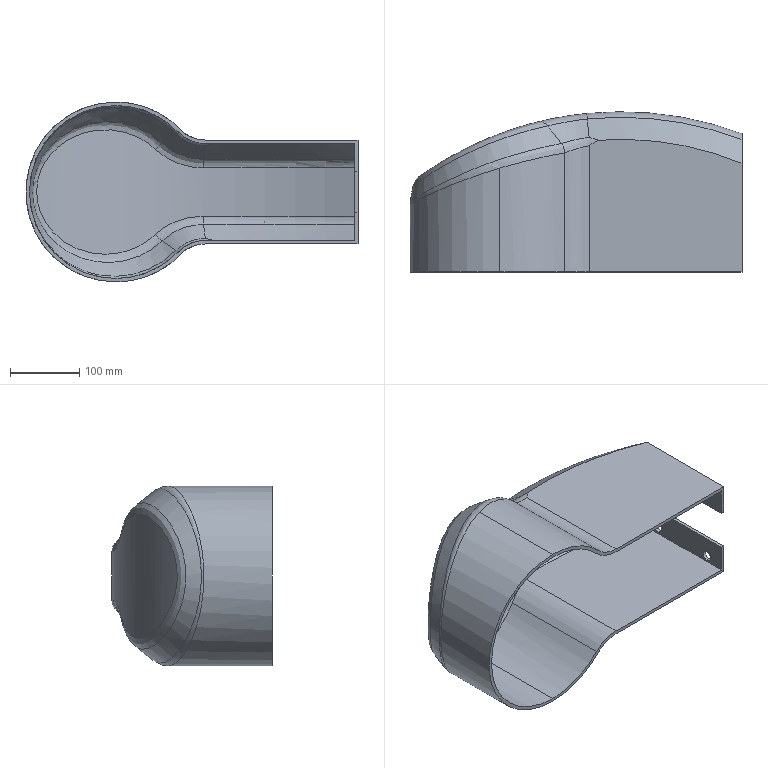Part | SolidWorks | features Fillet 2, ICE 2, Chamfer 1, Extrusion 1, Shell 1 | 1 solid | 56 faces | box 480 x 231.625 x 260 mm | volume 1531770 mm3 | cylinder 20 | spline 18 | plane 10 | cone 4 | torus 4 | commonest cylinder face diameters 15 x8 250 x3 260 x3 100 x2 110 x2 990 x1